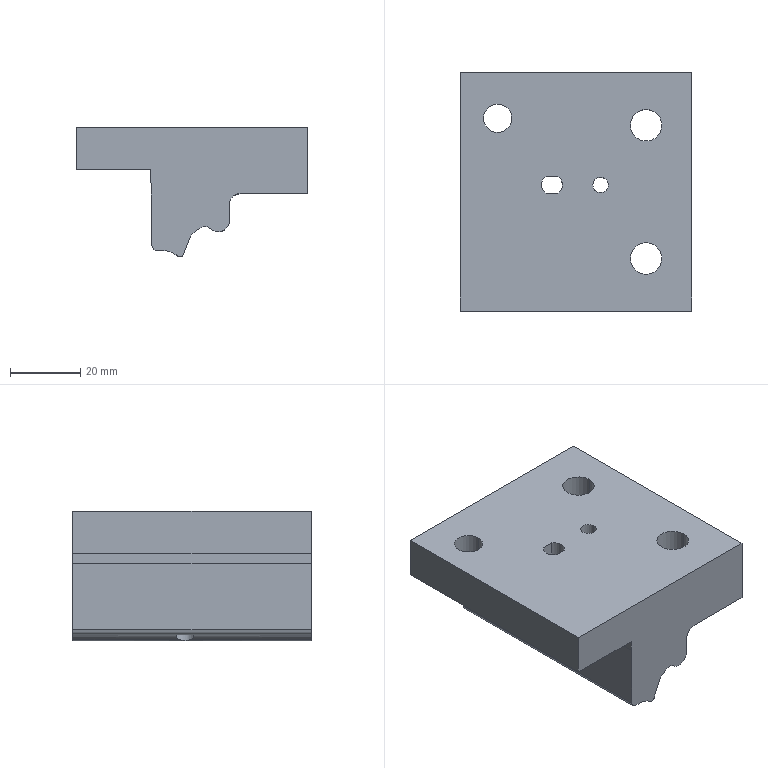Part | 1 solid | 47 faces | box 66.004 x 68 x 37.027 mm | volume 87960 mm3 | cylinder 25 | plane 22 | commonest cylinder face diameters 6 x4 9 x4 16 x4 4.415 x2 6.401 x2 8.1 x2